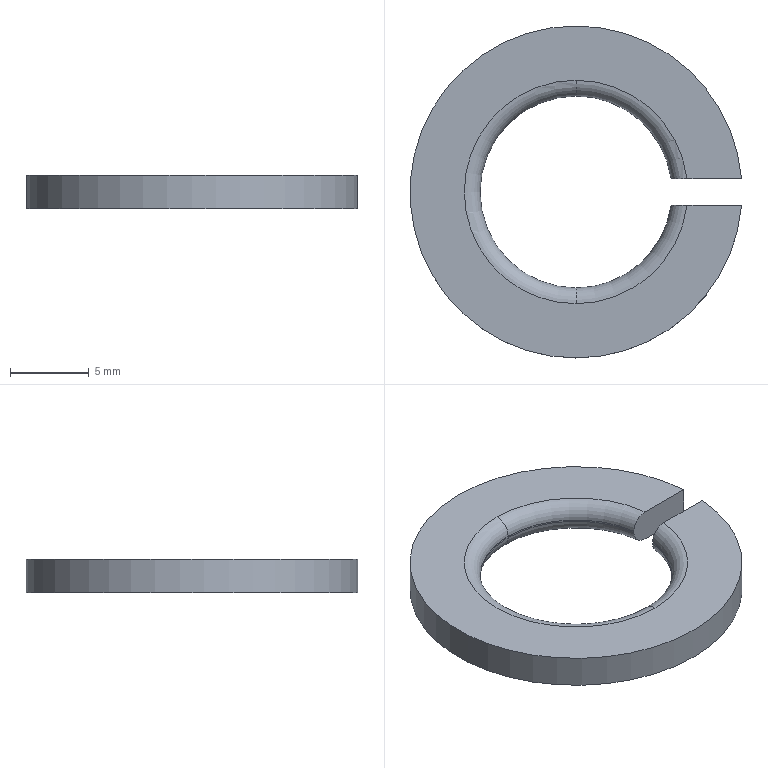Part | STEP file | Microwave Drying Flat Conveyor-din_128_a12 | 1 solid | 14 faces | box 21.067 x 21.1 x 2.1 mm | volume 456.756 mm3 | torus 6 | cylinder 4 | plane 4 | commonest cylinder face diameters 12.2 x3 21.1 x1
STEP:
#1=CARTESIAN_POINT('',(0.,-6.1,1.1));
#2=VERTEX_POINT('',#1);
#3=CARTESIAN_POINT('',(0.,6.1,1.1));
#4=VERTEX_POINT('',#3);
#5=CARTESIAN_POINT('',(0.,0.,1.1));
#6=DIRECTION('',(0.,0.,-1.));
#7=DIRECTION('',(0.,1.,0.));
#8=AXIS2_PLACEMENT_3D('',#5,#6,#7);
#9=CIRCLE('',#8,6.1);
#10=EDGE_CURVE('',#2,#4,#9,.T.);
#11=ORIENTED_EDGE('',*,*,#10,.F.);
#12=CARTESIAN_POINT('',(0.,-6.1,1.));
#13=VERTEX_POINT('',#12);
#14=CARTESIAN_POINT('',(0.,-6.1,0.));
#15=DIRECTION('',(0.,0.,-1.));
#16=VECTOR('',#15,1000.);
#17=LINE('',#14,#16);
#18=EDGE_CURVE('',#2,#13,#17,.T.);
#19=ORIENTED_EDGE('',*,*,#18,.T.);
#20=CARTESIAN_POINT('',(0.,6.1,1.));
#21=VERTEX_POINT('',#20);
#22=CARTESIAN_POINT('',(0.,0.,1.));
#23=DIRECTION('',(0.,0.,-1.));
#24=DIRECTION('',(0.,1.,0.));
#25=AXIS2_PLACEMENT_3D('',#22,#23,#24);
#26=CIRCLE('',#25,6.1);
#27=EDGE_CURVE('',#13,#21,#26,.T.);
#28=ORIENTED_EDGE('',*,*,#27,.T.);
#29=CARTESIAN_POINT('',(0.,6.1,0.));
#30=DIRECTION('',(0.,0.,-1.));
#31=VECTOR('',#30,1000.);
#32=LINE('',#29,#31);
#33=EDGE_CURVE('',#4,#21,#32,.T.);
#34=ORIENTED_EDGE('',*,*,#33,.F.);
#35=EDGE_LOOP('',(#11,#19,#28,#34));
#36=FACE_OUTER_BOUND('',#35,.T.);
#37=CARTESIAN_POINT('',(0.,0.,0.));
#38=DIRECTION('',(0.,0.,-1.));
#39=DIRECTION('',(0.,1.,0.));
#40=AXIS2_PLACEMENT_3D('',#37,#38,#39);
#41=CYLINDRICAL_SURFACE('',#40,6.1);
#42=ADVANCED_FACE('',(#36),#41,.F.);
#43=CARTESIAN_POINT('',(6.042,0.84,1.1));
#44=VERTEX_POINT('',#43);
#45=CARTESIAN_POINT('',(0.,0.,1.1));
#46=DIRECTION('',(0.,0.,-1.));
#47=DIRECTION('',(0.,1.,0.));
#48=AXIS2_PLACEMENT_3D('',#45,#46,#47);
#49=CIRCLE('',#48,6.1);
#50=EDGE_CURVE('',#4,#44,#49,.T.);
#51=ORIENTED_EDGE('',*,*,#50,.F.);
#52=ORIENTED_EDGE('',*,*,#33,.T.);
#53=CARTESIAN_POINT('',(6.042,0.84,1.));
#54=VERTEX_POINT('',#53);
#55=CARTESIAN_POINT('',(0.,0.,1.));
#56=DIRECTION('',(0.,0.,-1.));
#57=DIRECTION('',(0.,1.,0.));
#58=AXIS2_PLACEMENT_3D('',#55,#56,#57);
#59=CIRCLE('',#58,6.1);
#60=EDGE_CURVE('',#21,#54,#59,.T.);
#61=ORIENTED_EDGE('',*,*,#60,.T.);
#62=CARTESIAN_POINT('',(6.042,0.84,0.));
#63=DIRECTION('',(0.,0.,1.));
#64=VECTOR('',#63,1000.);
#65=LINE('',#62,#64);
#66=EDGE_CURVE('',#54,#44,#65,.T.);
#67=ORIENTED_EDGE('',*,*,#66,.T.);
#68=EDGE_LOOP('',(#51,#52,#61,#67));
#69=FACE_OUTER_BOUND('',#68,.T.);
#70=CARTESIAN_POINT('',(0.,0.,0.));
#71=DIRECTION('',(0.,0.,-1.));
#72=DIRECTION('',(0.,1.,0.));
#73=AXIS2_PLACEMENT_3D('',#70,#71,#72);
#74=CYLINDRICAL_SURFACE('',#73,6.1);
#75=ADVANCED_FACE('',(#69),#74,.F.);
#76=CARTESIAN_POINT('',(6.042,-0.84,1.1));
#77=VERTEX_POINT('',#76);
#78=CARTESIAN_POINT('',(0.,0.,1.1));
#79=DIRECTION('',(0.,0.,-1.));
#80=DIRECTION('',(0.,1.,0.));
#81=AXIS2_PLACEMENT_3D('',#78,#79,#80);
#82=CIRCLE('',#81,6.1);
#83=EDGE_CURVE('',#77,#2,#82,.T.);
#84=ORIENTED_EDGE('',*,*,#83,.T.);
#85=CARTESIAN_POINT('',(0.,-7.1,2.1));
#86=VERTEX_POINT('',#85);
#87=CARTESIAN_POINT('',(0.,-7.1,1.1));
#88=DIRECTION('',(1.,0.,0.));
#89=DIRECTION('',(0.,1.,0.));
#90=AXIS2_PLACEMENT_3D('',#87,#88,#89);
#91=CIRCLE('',#90,1.);
#92=EDGE_CURVE('',#2,#86,#91,.T.);
#93=ORIENTED_EDGE('',*,*,#92,.T.);
#94=CARTESIAN_POINT('',(7.05,-0.84,2.1));
#95=VERTEX_POINT('',#94);
#96=CARTESIAN_POINT('',(0.,0.,2.1));
#97=DIRECTION('',(0.,0.,-1.));
#98=DIRECTION('',(0.,1.,0.));
#99=AXIS2_PLACEMENT_3D('',#96,#97,#98);
#100=CIRCLE('',#99,7.1);
#101=EDGE_CURVE('',#95,#86,#100,.T.);
#102=ORIENTED_EDGE('',*,*,#101,.F.);
#103=CARTESIAN_POINT('',(7.05,-0.84,2.1));
#104=CARTESIAN_POINT('',(6.918,-0.84,2.1));
#105=CARTESIAN_POINT('',(6.787,-0.84,2.074));
#106=CARTESIAN_POINT('',(6.545,-0.84,1.975));
#107=CARTESIAN_POINT('',(6.432,-0.84,1.901));
#108=CARTESIAN_POINT('',(6.246,-0.84,1.717));
#109=CARTESIAN_POINT('',(6.171,-0.84,1.606));
#110=CARTESIAN_POINT('',(6.068,-0.84,1.362));
#111=CARTESIAN_POINT('',(6.042,-0.84,1.232));
#112=CARTESIAN_POINT('',(6.042,-0.84,1.1));
#113=B_SPLINE_CURVE_WITH_KNOTS('',3,(#103,#104,#105,#106,#107,#108,#109,#110,#111,#112),.UNSPECIFIED.,.F.,.F.,(4,2,2,2,4),(0.005077,0.005469,0.005862,0.006254,0.006646),.UNSPECIFIED.);
#114=EDGE_CURVE('',#95,#77,#113,.T.);
#115=ORIENTED_EDGE('',*,*,#114,.T.);
#116=EDGE_LOOP('',(#84,#93,#102,#115));
#117=FACE_OUTER_BOUND('',#116,.T.);
#118=CARTESIAN_POINT('',(0.,0.,1.1));
#119=DIRECTION('',(0.,0.,-1.));
#120=DIRECTION('',(0.,1.,0.));
#121=AXIS2_PLACEMENT_3D('',#118,#119,#120);
#122=TOROIDAL_SURFACE('',#121,7.1,1.);
#123=ADVANCED_FACE('',(#117),#122,.T.);
#124=ORIENTED_EDGE('',*,*,#92,.F.);
#125=ORIENTED_EDGE('',*,*,#10,.T.);
#126=CARTESIAN_POINT('',(0.,7.1,2.1));
#127=VERTEX_POINT('',#126);
#128=CARTESIAN_POINT('',(0.,7.1,1.1));
#129=DIRECTION('',(-1.,0.,0.));
#130=DIRECTION('',(0.,0.,1.));
#131=AXIS2_PLACEMENT_3D('',#128,#129,#130);
#132=CIRCLE('',#131,1.);
#133=EDGE_CURVE('',#4,#127,#132,.T.);
#134=ORIENTED_EDGE('',*,*,#133,.T.);
#135=CARTESIAN_POINT('',(0.,0.,2.1));
#136=DIRECTION('',(0.,0.,-1.));
#137=DIRECTION('',(0.,1.,0.));
#138=AXIS2_PLACEMENT_3D('',#135,#136,#137);
#139=CIRCLE('',#138,7.1);
#140=EDGE_CURVE('',#86,#127,#139,.T.);
#141=ORIENTED_EDGE('',*,*,#140,.F.);
#142=EDGE_LOOP('',(#124,#125,#134,#141));
#143=FACE_OUTER_BOUND('',#142,.T.);
#144=CARTESIAN_POINT('',(0.,0.,1.1));
#145=DIRECTION('',(0.,0.,-1.));
#146=DIRECTION('',(0.,1.,0.));
#147=AXIS2_PLACEMENT_3D('',#144,#145,#146);
#148=TOROIDAL_SURFACE('',#147,7.1,1.);
#149=ADVANCED_FACE('',(#143),#148,.T.);
#150=CARTESIAN_POINT('',(7.05,-0.84,0.));
#151=VERTEX_POINT('',#150);
#152=CARTESIAN_POINT('',(0.,-7.1,0.));
#153=VERTEX_POINT('',#152);
#154=CARTESIAN_POINT('',(0.,0.,0.));
#155=DIRECTION('',(0.,0.,-1.));
#156=DIRECTION('',(0.,1.,0.));
#157=AXIS2_PLACEMENT_3D('',#154,#155,#156);
#158=CIRCLE('',#157,7.1);
#159=EDGE_CURVE('',#151,#153,#158,.T.);
#160=ORIENTED_EDGE('',*,*,#159,.T.);
#161=CARTESIAN_POINT('',(0.,-7.1,1.));
#162=DIRECTION('',(1.,0.,0.));
#163=DIRECTION('',(0.,1.,0.));
#164=AXIS2_PLACEMENT_3D('',#161,#162,#163);
#165=CIRCLE('',#164,1.);
#166=EDGE_CURVE('',#153,#13,#165,.T.);
#167=ORIENTED_EDGE('',*,*,#166,.T.);
#168=CARTESIAN_POINT('',(6.042,-0.84,1.));
#169=VERTEX_POINT('',#168);
#170=CARTESIAN_POINT('',(0.,0.,1.));
#171=DIRECTION('',(0.,0.,-1.));
#172=DIRECTION('',(0.,1.,0.));
#173=AXIS2_PLACEMENT_3D('',#170,#171,#172);
#174=CIRCLE('',#173,6.1);
#175=EDGE_CURVE('',#169,#13,#174,.T.);
#176=ORIENTED_EDGE('',*,*,#175,.F.);
#177=CARTESIAN_POINT('',(6.042,-0.84,1.));
#178=CARTESIAN_POINT('',(6.042,-0.84,0.8693));
#179=CARTESIAN_POINT('',(6.068,-0.84,0.7367));
#180=CARTESIAN_POINT('',(6.171,-0.84,0.4932));
#181=CARTESIAN_POINT('',(6.246,-0.84,0.383));
#182=CARTESIAN_POINT('',(6.433,-0.84,0.1988));
#183=CARTESIAN_POINT('',(6.545,-0.84,0.125));
#184=CARTESIAN_POINT('',(6.787,-0.84,0.02595));
#185=CARTESIAN_POINT('',(6.919,-0.84,0.));
#186=CARTESIAN_POINT('',(7.05,-0.84,0.));
#187=B_SPLINE_CURVE_WITH_KNOTS('',3,(#177,#178,#179,#180,#181,#182,#183,#184,#185,#186),.UNSPECIFIED.,.F.,.F.,(4,2,2,2,4),(0.005905,0.006297,0.006689,0.007081,0.007473),.UNSPECIFIED.);
#188=EDGE_CURVE('',#169,#151,#187,.T.);
#189=ORIENTED_EDGE('',*,*,#188,.T.);
#190=EDGE_LOOP('',(#160,#167,#176,#189));
#191=FACE_OUTER_BOUND('',#190,.T.);
#192=CARTESIAN_POINT('',(0.,0.,1.));
#193=DIRECTION('',(0.,0.,-1.));
#194=DIRECTION('',(0.,1.,0.));
#195=AXIS2_PLACEMENT_3D('',#192,#193,#194);
#196=TOROIDAL_SURFACE('',#195,7.1,1.);
#197=ADVANCED_FACE('',(#191),#196,.T.);
#198=ORIENTED_EDGE('',*,*,#166,.F.);
#199=CARTESIAN_POINT('',(0.,7.1,0.));
#200=VERTEX_POINT('',#199);
#201=CARTESIAN_POINT('',(0.,0.,0.));
#202=DIRECTION('',(0.,0.,-1.));
#203=DIRECTION('',(0.,1.,0.));
#204=AXIS2_PLACEMENT_3D('',#201,#202,#203);
#205=CIRCLE('',#204,7.1);
#206=EDGE_CURVE('',#153,#200,#205,.T.);
#207=ORIENTED_EDGE('',*,*,#206,.T.);
#208=CARTESIAN_POINT('',(0.,7.1,1.));
#209=DIRECTION('',(-1.,0.,0.));
#210=DIRECTION('',(0.,0.,1.));
#211=AXIS2_PLACEMENT_3D('',#208,#209,#210);
#212=CIRCLE('',#211,1.);
#213=EDGE_CURVE('',#200,#21,#212,.T.);
#214=ORIENTED_EDGE('',*,*,#213,.T.);
#215=ORIENTED_EDGE('',*,*,#27,.F.);
#216=EDGE_LOOP('',(#198,#207,#214,#215));
#217=FACE_OUTER_BOUND('',#216,.T.);
#218=CARTESIAN_POINT('',(0.,0.,1.));
#219=DIRECTION('',(0.,0.,-1.));
#220=DIRECTION('',(0.,1.,0.));
#221=AXIS2_PLACEMENT_3D('',#218,#219,#220);
#222=TOROIDAL_SURFACE('',#221,7.1,1.);
#223=ADVANCED_FACE('',(#217),#222,.T.);
#224=CARTESIAN_POINT('',(10.517,-0.84,0.));
#225=VERTEX_POINT('',#224);
#226=CARTESIAN_POINT('',(0.,-0.84,0.));
#227=DIRECTION('',(-1.,0.,0.));
#228=VECTOR('',#227,1000.);
#229=LINE('',#226,#228);
#230=EDGE_CURVE('',#225,#151,#229,.T.);
#231=ORIENTED_EDGE('',*,*,#230,.F.);
#232=CARTESIAN_POINT('',(10.517,0.84,0.));
#233=VERTEX_POINT('',#232);
#234=CARTESIAN_POINT('',(0.,0.,0.));
#235=DIRECTION('',(0.,0.,1.));
#236=DIRECTION('',(1.,0.,0.));
#237=AXIS2_PLACEMENT_3D('',#234,#235,#236);
#238=CIRCLE('',#237,10.55);
#239=EDGE_CURVE('',#233,#225,#238,.T.);
#240=ORIENTED_EDGE('',*,*,#239,.F.);
#241=CARTESIAN_POINT('',(7.05,0.84,0.));
#242=VERTEX_POINT('',#241);
#243=CARTESIAN_POINT('',(0.,0.84,0.));
#244=DIRECTION('',(1.,0.,0.));
#245=VECTOR('',#244,1000.);
#246=LINE('',#243,#245);
#247=EDGE_CURVE('',#242,#233,#246,.T.);
#248=ORIENTED_EDGE('',*,*,#247,.F.);
#249=CARTESIAN_POINT('',(0.,0.,0.));
#250=DIRECTION('',(0.,0.,-1.));
#251=DIRECTION('',(0.,1.,0.));
#252=AXIS2_PLACEMENT_3D('',#249,#250,#251);
#253=CIRCLE('',#252,7.1);
#254=EDGE_CURVE('',#200,#242,#253,.T.);
#255=ORIENTED_EDGE('',*,*,#254,.F.);
#256=ORIENTED_EDGE('',*,*,#206,.F.);
#257=ORIENTED_EDGE('',*,*,#159,.F.);
#258=EDGE_LOOP('',(#231,#240,#248,#255,#256,#257));
#259=FACE_OUTER_BOUND('',#258,.T.);
#260=CARTESIAN_POINT('',(0.,0.,0.));
#261=DIRECTION('',(0.,0.,-1.));
#262=DIRECTION('',(0.,1.,0.));
#263=AXIS2_PLACEMENT_3D('',#260,#261,#262);
#264=PLANE('',#263);
#265=ADVANCED_FACE('',(#259),#264,.T.);
#266=CARTESIAN_POINT('',(10.517,-0.84,2.1));
#267=VERTEX_POINT('',#266);
#268=CARTESIAN_POINT('',(0.,-0.84,2.1));
#269=DIRECTION('',(1.,0.,0.));
#270=VECTOR('',#269,1000.);
#271=LINE('',#268,#270);
#272=EDGE_CURVE('',#95,#267,#271,.T.);
#273=ORIENTED_EDGE('',*,*,#272,.F.);
#274=ORIENTED_EDGE('',*,*,#101,.T.);
#275=ORIENTED_EDGE('',*,*,#140,.T.);
#276=CARTESIAN_POINT('',(7.05,0.84,2.1));
#277=VERTEX_POINT('',#276);
#278=CARTESIAN_POINT('',(0.,0.,2.1));
#279=DIRECTION('',(0.,0.,-1.));
#280=DIRECTION('',(0.,1.,0.));
#281=AXIS2_PLACEMENT_3D('',#278,#279,#280);
#282=CIRCLE('',#281,7.1);
#283=EDGE_CURVE('',#127,#277,#282,.T.);
#284=ORIENTED_EDGE('',*,*,#283,.T.);
#285=CARTESIAN_POINT('',(10.517,0.84,2.1));
#286=VERTEX_POINT('',#285);
#287=CARTESIAN_POINT('',(0.,0.84,2.1));
#288=DIRECTION('',(-1.,0.,0.));
#289=VECTOR('',#288,1000.);
#290=LINE('',#287,#289);
#291=EDGE_CURVE('',#286,#277,#290,.T.);
#292=ORIENTED_EDGE('',*,*,#291,.F.);
#293=CARTESIAN_POINT('',(0.,0.,2.1));
#294=DIRECTION('',(0.,0.,-1.));
#295=DIRECTION('',(1.,0.,0.));
#296=AXIS2_PLACEMENT_3D('',#293,#294,#295);
#297=CIRCLE('',#296,10.55);
#298=EDGE_CURVE('',#267,#286,#297,.T.);
#299=ORIENTED_EDGE('',*,*,#298,.F.);
#300=EDGE_LOOP('',(#273,#274,#275,#284,#292,#299));
#301=FACE_OUTER_BOUND('',#300,.T.);
#302=CARTESIAN_POINT('',(0.,0.,2.1));
#303=DIRECTION('',(0.,0.,1.));
#304=DIRECTION('',(0.,-1.,0.));
#305=AXIS2_PLACEMENT_3D('',#302,#303,#304);
#306=PLANE('',#305);
#307=ADVANCED_FACE('',(#301),#306,.T.);
#308=CARTESIAN_POINT('',(10.517,-0.84,0.));
#309=DIRECTION('',(0.,0.,-1.));
#310=VECTOR('',#309,1000.);
#311=LINE('',#308,#310);
#312=EDGE_CURVE('',#267,#225,#311,.T.);
#313=ORIENTED_EDGE('',*,*,#312,.F.);
#314=ORIENTED_EDGE('',*,*,#298,.T.);
#315=CARTESIAN_POINT('',(10.517,0.84,0.));
#316=DIRECTION('',(0.,0.,1.));
#317=VECTOR('',#316,1000.);
#318=LINE('',#315,#317);
#319=EDGE_CURVE('',#233,#286,#318,.T.);
#320=ORIENTED_EDGE('',*,*,#319,.F.);
#321=ORIENTED_EDGE('',*,*,#239,.T.);
#322=EDGE_LOOP('',(#313,#314,#320,#321));
#323=FACE_OUTER_BOUND('',#322,.T.);
#324=CARTESIAN_POINT('',(0.,0.,0.));
#325=DIRECTION('',(0.,0.,1.));
#326=DIRECTION('',(1.,0.,0.));
#327=AXIS2_PLACEMENT_3D('',#324,#325,#326);
#328=CYLINDRICAL_SURFACE('',#327,10.55);
#329=ADVANCED_FACE('',(#323),#328,.T.);
#330=ORIENTED_EDGE('',*,*,#213,.F.);
#331=ORIENTED_EDGE('',*,*,#254,.T.);
#332=CARTESIAN_POINT('',(7.05,0.84,0.));
#333=CARTESIAN_POINT('',(6.918,0.84,0.));
#334=CARTESIAN_POINT('',(6.787,0.84,0.0259));
#335=CARTESIAN_POINT('',(6.545,0.84,0.1252));
#336=CARTESIAN_POINT('',(6.432,0.84,0.1992));
#337=CARTESIAN_POINT('',(6.246,0.84,0.3829));
#338=CARTESIAN_POINT('',(6.171,0.84,0.4939));
#339=CARTESIAN_POINT('',(6.068,0.84,0.7379));
#340=CARTESIAN_POINT('',(6.042,0.84,0.8682));
#341=CARTESIAN_POINT('',(6.042,0.84,1.));
#342=B_SPLINE_CURVE_WITH_KNOTS('',3,(#332,#333,#334,#335,#336,#337,#338,#339,#340,#341),.UNSPECIFIED.,.F.,.F.,(4,2,2,2,4),(0.005077,0.005469,0.005862,0.006254,0.006646),.UNSPECIFIED.);
#343=EDGE_CURVE('',#242,#54,#342,.T.);
#344=ORIENTED_EDGE('',*,*,#343,.T.);
#345=ORIENTED_EDGE('',*,*,#60,.F.);
#346=EDGE_LOOP('',(#330,#331,#344,#345));
#347=FACE_OUTER_BOUND('',#346,.T.);
#348=CARTESIAN_POINT('',(0.,0.,1.));
#349=DIRECTION('',(0.,0.,-1.));
#350=DIRECTION('',(0.,1.,0.));
#351=AXIS2_PLACEMENT_3D('',#348,#349,#350);
#352=TOROIDAL_SURFACE('',#351,7.1,1.);
#353=ADVANCED_FACE('',(#347),#352,.T.);
#354=ORIENTED_EDGE('',*,*,#133,.F.);
#355=ORIENTED_EDGE('',*,*,#50,.T.);
#356=CARTESIAN_POINT('',(6.042,0.84,1.1));
#357=CARTESIAN_POINT('',(6.042,0.84,1.231));
#358=CARTESIAN_POINT('',(6.068,0.84,1.363));
#359=CARTESIAN_POINT('',(6.171,0.84,1.607));
#360=CARTESIAN_POINT('',(6.246,0.84,1.717));
#361=CARTESIAN_POINT('',(6.433,0.84,1.901));
#362=CARTESIAN_POINT('',(6.545,0.84,1.975));
#363=CARTESIAN_POINT('',(6.787,0.84,2.074));
#364=CARTESIAN_POINT('',(6.919,0.84,2.1));
#365=CARTESIAN_POINT('',(7.05,0.84,2.1));
#366=B_SPLINE_CURVE_WITH_KNOTS('',3,(#356,#357,#358,#359,#360,#361,#362,#363,#364,#365),.UNSPECIFIED.,.F.,.F.,(4,2,2,2,4),(0.005905,0.006297,0.006689,0.007081,0.007473),.UNSPECIFIED.);
#367=EDGE_CURVE('',#44,#277,#366,.T.);
#368=ORIENTED_EDGE('',*,*,#367,.T.);
#369=ORIENTED_EDGE('',*,*,#283,.F.);
#370=EDGE_LOOP('',(#354,#355,#368,#369));
#371=FACE_OUTER_BOUND('',#370,.T.);
#372=CARTESIAN_POINT('',(0.,0.,1.1));
#373=DIRECTION('',(0.,0.,-1.));
#374=DIRECTION('',(0.,1.,0.));
#375=AXIS2_PLACEMENT_3D('',#372,#373,#374);
#376=TOROIDAL_SURFACE('',#375,7.1,1.);
#377=ADVANCED_FACE('',(#371),#376,.T.);
#378=ORIENTED_EDGE('',*,*,#18,.F.);
#379=ORIENTED_EDGE('',*,*,#83,.F.);
#380=CARTESIAN_POINT('',(6.042,-0.84,0.));
#381=DIRECTION('',(0.,0.,-1.));
#382=VECTOR('',#381,1000.);
#383=LINE('',#380,#382);
#384=EDGE_CURVE('',#77,#169,#383,.T.);
#385=ORIENTED_EDGE('',*,*,#384,.T.);
#386=ORIENTED_EDGE('',*,*,#175,.T.);
#387=EDGE_LOOP('',(#378,#379,#385,#386));
#388=FACE_OUTER_BOUND('',#387,.T.);
#389=CARTESIAN_POINT('',(0.,0.,0.));
#390=DIRECTION('',(0.,0.,-1.));
#391=DIRECTION('',(0.,1.,0.));
#392=AXIS2_PLACEMENT_3D('',#389,#390,#391);
#393=CYLINDRICAL_SURFACE('',#392,6.1);
#394=ADVANCED_FACE('',(#388),#393,.F.);
#395=ORIENTED_EDGE('',*,*,#319,.T.);
#396=ORIENTED_EDGE('',*,*,#291,.T.);
#397=ORIENTED_EDGE('',*,*,#367,.F.);
#398=ORIENTED_EDGE('',*,*,#66,.F.);
#399=ORIENTED_EDGE('',*,*,#343,.F.);
#400=ORIENTED_EDGE('',*,*,#247,.T.);
#401=EDGE_LOOP('',(#395,#396,#397,#398,#399,#400));
#402=FACE_OUTER_BOUND('',#401,.T.);
#403=CARTESIAN_POINT('',(10.55,0.84,1.05));
#404=DIRECTION('',(0.,1.,0.));
#405=DIRECTION('',(-1.,0.,0.));
#406=AXIS2_PLACEMENT_3D('',#403,#404,#405);
#407=PLANE('',#406);
#408=ADVANCED_FACE('',(#402),#407,.F.);
#409=ORIENTED_EDGE('',*,*,#312,.T.);
#410=ORIENTED_EDGE('',*,*,#230,.T.);
#411=ORIENTED_EDGE('',*,*,#188,.F.);
#412=ORIENTED_EDGE('',*,*,#384,.F.);
#413=ORIENTED_EDGE('',*,*,#114,.F.);
#414=ORIENTED_EDGE('',*,*,#272,.T.);
#415=EDGE_LOOP('',(#409,#410,#411,#412,#413,#414));
#416=FACE_OUTER_BOUND('',#415,.T.);
#417=CARTESIAN_POINT('',(10.55,-0.84,1.05));
#418=DIRECTION('',(0.,-1.,0.));
#419=DIRECTION('',(1.,0.,0.));
#420=AXIS2_PLACEMENT_3D('',#417,#418,#419);
#421=PLANE('',#420);
#422=ADVANCED_FACE('',(#416),#421,.F.);
#423=CLOSED_SHELL('',(#42,#75,#123,#149,#197,#223,#265,#307,#329,#353,#377,#394,#408,#422));
#424=MANIFOLD_SOLID_BREP('',#423);
#425=CARTESIAN_POINT('',(0.,0.,0.));
#426=DIRECTION('',(0.,0.,1.));
#427=DIRECTION('',(1.,0.,0.));
#428=AXIS2_PLACEMENT_3D('',#425,#426,#427);
#429=(LENGTH_UNIT()NAMED_UNIT(*)SI_UNIT(.MILLI.,.METRE.));
#430=UNCERTAINTY_MEASURE_WITH_UNIT(LENGTH_MEASURE(0.00001),#429,'','');
#431=(NAMED_UNIT(*)PLANE_ANGLE_UNIT()SI_UNIT($,.RADIAN.));
#432=(NAMED_UNIT(*)SI_UNIT($,.STERADIAN.)SOLID_ANGLE_UNIT());
#433=(GEOMETRIC_REPRESENTATION_CONTEXT(3)GLOBAL_UNCERTAINTY_ASSIGNED_CONTEXT((#430))GLOBAL_UNIT_ASSIGNED_CONTEXT((#429,#431,#432))REPRESENTATION_CONTEXT('',''));
#434=ADVANCED_BREP_SHAPE_REPRESENTATION('',(#424,#428),#433);